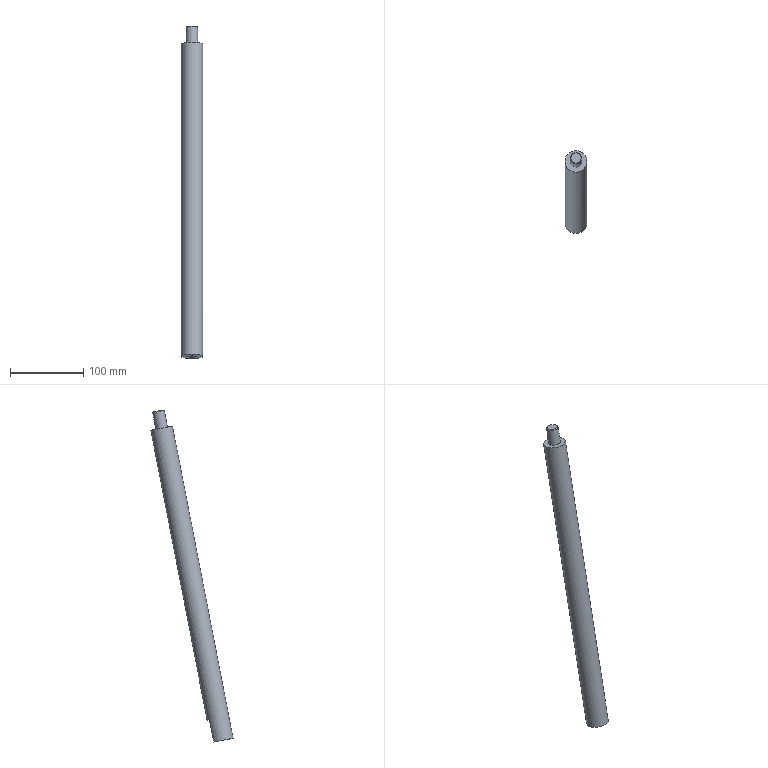Part | STEP file | solid 104 | 1 solid | 11 faces | box 30 x 112.165 x 452.721 mm | volume 308363 mm3 | plane 5 | cylinder 3 | cone 3 | commonest cylinder face diameters 10.2 x1 16 x1 30 x1